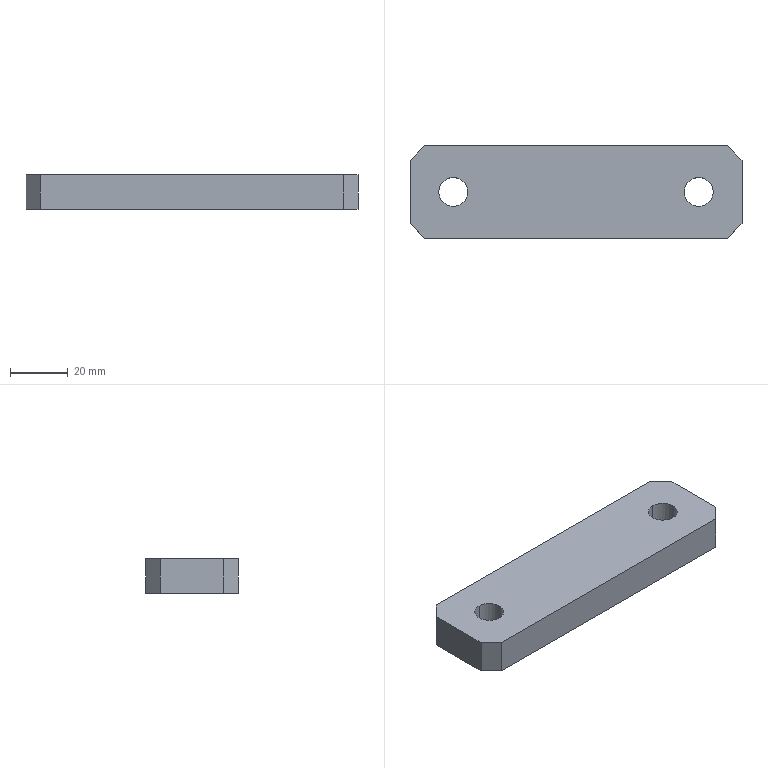Part | STEP file | [23] | 1 solid | 14 faces | box 115 x 32 x 12 mm | volume 41675 mm3 | plane 10 | cylinder 4 | commonest cylinder face diameters 10 x4
STEP:
#1=CARTESIAN_POINT('',(61.,21.,12.));
#2=VERTEX_POINT('',#1);
#3=CARTESIAN_POINT('',(61.,11.,12.));
#4=VERTEX_POINT('',#3);
#5=CARTESIAN_POINT('',(61.,16.,12.));
#6=DIRECTION('',(0.,0.,-1.));
#7=DIRECTION('',(0.,-1.,0.));
#8=AXIS2_PLACEMENT_3D('',#5,#6,#7);
#9=CIRCLE('',#8,5.);
#10=EDGE_CURVE('',#2,#4,#9,.T.);
#11=ORIENTED_EDGE('',*,*,#10,.F.);
#12=CARTESIAN_POINT('',(61.,21.,0.));
#13=VERTEX_POINT('',#12);
#14=CARTESIAN_POINT('',(61.,21.,12.));
#15=DIRECTION('',(0.,0.,-1.));
#16=VECTOR('',#15,1000.);
#17=LINE('',#14,#16);
#18=EDGE_CURVE('',#2,#13,#17,.T.);
#19=ORIENTED_EDGE('',*,*,#18,.T.);
#20=CARTESIAN_POINT('',(61.,11.,0.));
#21=VERTEX_POINT('',#20);
#22=CARTESIAN_POINT('',(61.,16.,0.));
#23=DIRECTION('',(0.,0.,1.));
#24=DIRECTION('',(0.,1.,0.));
#25=AXIS2_PLACEMENT_3D('',#22,#23,#24);
#26=CIRCLE('',#25,5.);
#27=EDGE_CURVE('',#21,#13,#26,.T.);
#28=ORIENTED_EDGE('',*,*,#27,.F.);
#29=CARTESIAN_POINT('',(61.,11.,12.));
#30=DIRECTION('',(0.,0.,-1.));
#31=VECTOR('',#30,1000.);
#32=LINE('',#29,#31);
#33=EDGE_CURVE('',#4,#21,#32,.T.);
#34=ORIENTED_EDGE('',*,*,#33,.F.);
#35=EDGE_LOOP('',(#11,#19,#28,#34));
#36=FACE_OUTER_BOUND('',#35,.T.);
#37=CARTESIAN_POINT('',(61.,16.,12.));
#38=DIRECTION('',(0.,0.,-1.));
#39=DIRECTION('',(0.,-1.,0.));
#40=AXIS2_PLACEMENT_3D('',#37,#38,#39);
#41=CYLINDRICAL_SURFACE('',#40,5.);
#42=ADVANCED_FACE('',(#36),#41,.F.);
#43=CARTESIAN_POINT('',(-24.,21.,12.));
#44=VERTEX_POINT('',#43);
#45=CARTESIAN_POINT('',(-24.,11.,12.));
#46=VERTEX_POINT('',#45);
#47=CARTESIAN_POINT('',(-24.,16.,12.));
#48=DIRECTION('',(0.,0.,-1.));
#49=DIRECTION('',(0.,-1.,0.));
#50=AXIS2_PLACEMENT_3D('',#47,#48,#49);
#51=CIRCLE('',#50,5.);
#52=EDGE_CURVE('',#44,#46,#51,.T.);
#53=ORIENTED_EDGE('',*,*,#52,.F.);
#54=CARTESIAN_POINT('',(-24.,21.,0.));
#55=VERTEX_POINT('',#54);
#56=CARTESIAN_POINT('',(-24.,21.,12.));
#57=DIRECTION('',(0.,0.,-1.));
#58=VECTOR('',#57,1000.);
#59=LINE('',#56,#58);
#60=EDGE_CURVE('',#44,#55,#59,.T.);
#61=ORIENTED_EDGE('',*,*,#60,.T.);
#62=CARTESIAN_POINT('',(-24.,11.,0.));
#63=VERTEX_POINT('',#62);
#64=CARTESIAN_POINT('',(-24.,16.,0.));
#65=DIRECTION('',(0.,0.,1.));
#66=DIRECTION('',(0.,1.,0.));
#67=AXIS2_PLACEMENT_3D('',#64,#65,#66);
#68=CIRCLE('',#67,5.);
#69=EDGE_CURVE('',#63,#55,#68,.T.);
#70=ORIENTED_EDGE('',*,*,#69,.F.);
#71=CARTESIAN_POINT('',(-24.,11.,12.));
#72=DIRECTION('',(0.,0.,-1.));
#73=VECTOR('',#72,1000.);
#74=LINE('',#71,#73);
#75=EDGE_CURVE('',#46,#63,#74,.T.);
#76=ORIENTED_EDGE('',*,*,#75,.F.);
#77=EDGE_LOOP('',(#53,#61,#70,#76));
#78=FACE_OUTER_BOUND('',#77,.T.);
#79=CARTESIAN_POINT('',(-24.,16.,12.));
#80=DIRECTION('',(0.,0.,-1.));
#81=DIRECTION('',(0.,-1.,0.));
#82=AXIS2_PLACEMENT_3D('',#79,#80,#81);
#83=CYLINDRICAL_SURFACE('',#82,5.);
#84=ADVANCED_FACE('',(#78),#83,.F.);
#85=CARTESIAN_POINT('',(61.,16.,12.));
#86=DIRECTION('',(0.,0.,-1.));
#87=DIRECTION('',(0.,-1.,0.));
#88=AXIS2_PLACEMENT_3D('',#85,#86,#87);
#89=CIRCLE('',#88,5.);
#90=EDGE_CURVE('',#4,#2,#89,.T.);
#91=ORIENTED_EDGE('',*,*,#90,.T.);
#92=ORIENTED_EDGE('',*,*,#10,.T.);
#93=EDGE_LOOP('',(#91,#92));
#94=FACE_BOUND('',#93,.T.);
#95=CARTESIAN_POINT('',(-24.,16.,12.));
#96=DIRECTION('',(0.,0.,-1.));
#97=DIRECTION('',(0.,-1.,0.));
#98=AXIS2_PLACEMENT_3D('',#95,#96,#97);
#99=CIRCLE('',#98,5.);
#100=EDGE_CURVE('',#46,#44,#99,.T.);
#101=ORIENTED_EDGE('',*,*,#100,.T.);
#102=ORIENTED_EDGE('',*,*,#52,.T.);
#103=EDGE_LOOP('',(#101,#102));
#104=FACE_BOUND('',#103,.T.);
#105=CARTESIAN_POINT('',(71.,0.,12.));
#106=VERTEX_POINT('',#105);
#107=CARTESIAN_POINT('',(-34.,0.,12.));
#108=VERTEX_POINT('',#107);
#109=CARTESIAN_POINT('',(18.5,0.,12.));
#110=DIRECTION('',(-1.,0.,0.));
#111=VECTOR('',#110,1000.);
#112=LINE('',#109,#111);
#113=EDGE_CURVE('',#106,#108,#112,.T.);
#114=ORIENTED_EDGE('',*,*,#113,.F.);
#115=CARTESIAN_POINT('',(76.,5.,12.));
#116=VERTEX_POINT('',#115);
#117=CARTESIAN_POINT('',(52.75,-18.25,12.));
#118=DIRECTION('',(0.7071,0.7071,0.));
#119=VECTOR('',#118,1000.);
#120=LINE('',#117,#119);
#121=EDGE_CURVE('',#106,#116,#120,.T.);
#122=ORIENTED_EDGE('',*,*,#121,.T.);
#123=CARTESIAN_POINT('',(76.,27.,12.));
#124=VERTEX_POINT('',#123);
#125=CARTESIAN_POINT('',(76.,16.,12.));
#126=DIRECTION('',(0.,-1.,0.));
#127=VECTOR('',#126,1000.);
#128=LINE('',#125,#127);
#129=EDGE_CURVE('',#124,#116,#128,.T.);
#130=ORIENTED_EDGE('',*,*,#129,.F.);
#131=CARTESIAN_POINT('',(71.,32.,12.));
#132=VERTEX_POINT('',#131);
#133=CARTESIAN_POINT('',(52.75,50.25,12.));
#134=DIRECTION('',(-0.7071,0.7071,0.));
#135=VECTOR('',#134,1000.);
#136=LINE('',#133,#135);
#137=EDGE_CURVE('',#124,#132,#136,.T.);
#138=ORIENTED_EDGE('',*,*,#137,.T.);
#139=CARTESIAN_POINT('',(-34.,32.,12.));
#140=VERTEX_POINT('',#139);
#141=CARTESIAN_POINT('',(18.5,32.,12.));
#142=DIRECTION('',(1.,0.,0.));
#143=VECTOR('',#142,1000.);
#144=LINE('',#141,#143);
#145=EDGE_CURVE('',#140,#132,#144,.T.);
#146=ORIENTED_EDGE('',*,*,#145,.F.);
#147=CARTESIAN_POINT('',(-39.,27.,12.));
#148=VERTEX_POINT('',#147);
#149=CARTESIAN_POINT('',(-15.75,50.25,12.));
#150=DIRECTION('',(-0.7071,-0.7071,0.));
#151=VECTOR('',#150,1000.);
#152=LINE('',#149,#151);
#153=EDGE_CURVE('',#140,#148,#152,.T.);
#154=ORIENTED_EDGE('',*,*,#153,.T.);
#155=CARTESIAN_POINT('',(-39.,5.,12.));
#156=VERTEX_POINT('',#155);
#157=CARTESIAN_POINT('',(-39.,16.,12.));
#158=DIRECTION('',(0.,1.,0.));
#159=VECTOR('',#158,1000.);
#160=LINE('',#157,#159);
#161=EDGE_CURVE('',#156,#148,#160,.T.);
#162=ORIENTED_EDGE('',*,*,#161,.F.);
#163=CARTESIAN_POINT('',(-15.75,-18.25,12.));
#164=DIRECTION('',(0.7071,-0.7071,0.));
#165=VECTOR('',#164,1000.);
#166=LINE('',#163,#165);
#167=EDGE_CURVE('',#156,#108,#166,.T.);
#168=ORIENTED_EDGE('',*,*,#167,.T.);
#169=EDGE_LOOP('',(#114,#122,#130,#138,#146,#154,#162,#168));
#170=FACE_OUTER_BOUND('',#169,.T.);
#171=CARTESIAN_POINT('',(18.5,16.,12.));
#172=DIRECTION('',(0.,0.,1.));
#173=DIRECTION('',(0.,1.,0.));
#174=AXIS2_PLACEMENT_3D('',#171,#172,#173);
#175=PLANE('',#174);
#176=ADVANCED_FACE('',(#94,#104,#170),#175,.T.);
#177=ORIENTED_EDGE('',*,*,#129,.T.);
#178=CARTESIAN_POINT('',(76.,5.,0.));
#179=VERTEX_POINT('',#178);
#180=CARTESIAN_POINT('',(76.,5.,0.));
#181=DIRECTION('',(0.,0.,-1.));
#182=VECTOR('',#181,1000.);
#183=LINE('',#180,#182);
#184=EDGE_CURVE('',#116,#179,#183,.T.);
#185=ORIENTED_EDGE('',*,*,#184,.T.);
#186=CARTESIAN_POINT('',(76.,27.,0.));
#187=VERTEX_POINT('',#186);
#188=CARTESIAN_POINT('',(76.,16.,0.));
#189=DIRECTION('',(0.,1.,0.));
#190=VECTOR('',#189,1000.);
#191=LINE('',#188,#190);
#192=EDGE_CURVE('',#179,#187,#191,.T.);
#193=ORIENTED_EDGE('',*,*,#192,.T.);
#194=CARTESIAN_POINT('',(76.,27.,0.));
#195=DIRECTION('',(0.,0.,1.));
#196=VECTOR('',#195,1000.);
#197=LINE('',#194,#196);
#198=EDGE_CURVE('',#187,#124,#197,.T.);
#199=ORIENTED_EDGE('',*,*,#198,.T.);
#200=EDGE_LOOP('',(#177,#185,#193,#199));
#201=FACE_OUTER_BOUND('',#200,.T.);
#202=CARTESIAN_POINT('',(76.,16.,0.));
#203=DIRECTION('',(1.,0.,0.));
#204=DIRECTION('',(0.,0.,-1.));
#205=AXIS2_PLACEMENT_3D('',#202,#203,#204);
#206=PLANE('',#205);
#207=ADVANCED_FACE('',(#201),#206,.T.);
#208=CARTESIAN_POINT('',(-34.,0.,0.));
#209=VERTEX_POINT('',#208);
#210=CARTESIAN_POINT('',(71.,0.,0.));
#211=VERTEX_POINT('',#210);
#212=CARTESIAN_POINT('',(18.5,0.,0.));
#213=DIRECTION('',(1.,0.,0.));
#214=VECTOR('',#213,1000.);
#215=LINE('',#212,#214);
#216=EDGE_CURVE('',#209,#211,#215,.T.);
#217=ORIENTED_EDGE('',*,*,#216,.T.);
#218=CARTESIAN_POINT('',(71.,0.,0.));
#219=DIRECTION('',(0.,0.,1.));
#220=VECTOR('',#219,1000.);
#221=LINE('',#218,#220);
#222=EDGE_CURVE('',#211,#106,#221,.T.);
#223=ORIENTED_EDGE('',*,*,#222,.T.);
#224=ORIENTED_EDGE('',*,*,#113,.T.);
#225=CARTESIAN_POINT('',(-34.,0.,0.));
#226=DIRECTION('',(0.,0.,-1.));
#227=VECTOR('',#226,1000.);
#228=LINE('',#225,#227);
#229=EDGE_CURVE('',#108,#209,#228,.T.);
#230=ORIENTED_EDGE('',*,*,#229,.T.);
#231=EDGE_LOOP('',(#217,#223,#224,#230));
#232=FACE_OUTER_BOUND('',#231,.T.);
#233=CARTESIAN_POINT('',(18.5,0.,0.));
#234=DIRECTION('',(0.,-1.,0.));
#235=DIRECTION('',(0.,0.,1.));
#236=AXIS2_PLACEMENT_3D('',#233,#234,#235);
#237=PLANE('',#236);
#238=ADVANCED_FACE('',(#232),#237,.T.);
#239=ORIENTED_EDGE('',*,*,#161,.T.);
#240=CARTESIAN_POINT('',(-39.,27.,0.));
#241=VERTEX_POINT('',#240);
#242=CARTESIAN_POINT('',(-39.,27.,0.));
#243=DIRECTION('',(0.,0.,-1.));
#244=VECTOR('',#243,1000.);
#245=LINE('',#242,#244);
#246=EDGE_CURVE('',#148,#241,#245,.T.);
#247=ORIENTED_EDGE('',*,*,#246,.T.);
#248=CARTESIAN_POINT('',(-39.,5.,0.));
#249=VERTEX_POINT('',#248);
#250=CARTESIAN_POINT('',(-39.,16.,0.));
#251=DIRECTION('',(0.,-1.,0.));
#252=VECTOR('',#251,1000.);
#253=LINE('',#250,#252);
#254=EDGE_CURVE('',#241,#249,#253,.T.);
#255=ORIENTED_EDGE('',*,*,#254,.T.);
#256=CARTESIAN_POINT('',(-39.,5.,0.));
#257=DIRECTION('',(0.,0.,1.));
#258=VECTOR('',#257,1000.);
#259=LINE('',#256,#258);
#260=EDGE_CURVE('',#249,#156,#259,.T.);
#261=ORIENTED_EDGE('',*,*,#260,.T.);
#262=EDGE_LOOP('',(#239,#247,#255,#261));
#263=FACE_OUTER_BOUND('',#262,.T.);
#264=CARTESIAN_POINT('',(-39.,16.,0.));
#265=DIRECTION('',(-1.,0.,0.));
#266=DIRECTION('',(0.,0.,1.));
#267=AXIS2_PLACEMENT_3D('',#264,#265,#266);
#268=PLANE('',#267);
#269=ADVANCED_FACE('',(#263),#268,.T.);
#270=ORIENTED_EDGE('',*,*,#27,.T.);
#271=CARTESIAN_POINT('',(61.,16.,0.));
#272=DIRECTION('',(0.,0.,1.));
#273=DIRECTION('',(0.,1.,0.));
#274=AXIS2_PLACEMENT_3D('',#271,#272,#273);
#275=CIRCLE('',#274,5.);
#276=EDGE_CURVE('',#13,#21,#275,.T.);
#277=ORIENTED_EDGE('',*,*,#276,.T.);
#278=EDGE_LOOP('',(#270,#277));
#279=FACE_BOUND('',#278,.T.);
#280=ORIENTED_EDGE('',*,*,#69,.T.);
#281=CARTESIAN_POINT('',(-24.,16.,0.));
#282=DIRECTION('',(0.,0.,1.));
#283=DIRECTION('',(0.,1.,0.));
#284=AXIS2_PLACEMENT_3D('',#281,#282,#283);
#285=CIRCLE('',#284,5.);
#286=EDGE_CURVE('',#55,#63,#285,.T.);
#287=ORIENTED_EDGE('',*,*,#286,.T.);
#288=EDGE_LOOP('',(#280,#287));
#289=FACE_BOUND('',#288,.T.);
#290=ORIENTED_EDGE('',*,*,#192,.F.);
#291=CARTESIAN_POINT('',(52.75,-18.25,0.));
#292=DIRECTION('',(-0.7071,-0.7071,0.));
#293=VECTOR('',#292,1000.);
#294=LINE('',#291,#293);
#295=EDGE_CURVE('',#179,#211,#294,.T.);
#296=ORIENTED_EDGE('',*,*,#295,.T.);
#297=ORIENTED_EDGE('',*,*,#216,.F.);
#298=CARTESIAN_POINT('',(-15.75,-18.25,0.));
#299=DIRECTION('',(-0.7071,0.7071,0.));
#300=VECTOR('',#299,1000.);
#301=LINE('',#298,#300);
#302=EDGE_CURVE('',#209,#249,#301,.T.);
#303=ORIENTED_EDGE('',*,*,#302,.T.);
#304=ORIENTED_EDGE('',*,*,#254,.F.);
#305=CARTESIAN_POINT('',(-34.,32.,0.));
#306=VERTEX_POINT('',#305);
#307=CARTESIAN_POINT('',(-15.75,50.25,0.));
#308=DIRECTION('',(0.7071,0.7071,0.));
#309=VECTOR('',#308,1000.);
#310=LINE('',#307,#309);
#311=EDGE_CURVE('',#241,#306,#310,.T.);
#312=ORIENTED_EDGE('',*,*,#311,.T.);
#313=CARTESIAN_POINT('',(71.,32.,0.));
#314=VERTEX_POINT('',#313);
#315=CARTESIAN_POINT('',(18.5,32.,0.));
#316=DIRECTION('',(-1.,0.,0.));
#317=VECTOR('',#316,1000.);
#318=LINE('',#315,#317);
#319=EDGE_CURVE('',#314,#306,#318,.T.);
#320=ORIENTED_EDGE('',*,*,#319,.F.);
#321=CARTESIAN_POINT('',(52.75,50.25,0.));
#322=DIRECTION('',(0.7071,-0.7071,0.));
#323=VECTOR('',#322,1000.);
#324=LINE('',#321,#323);
#325=EDGE_CURVE('',#314,#187,#324,.T.);
#326=ORIENTED_EDGE('',*,*,#325,.T.);
#327=EDGE_LOOP('',(#290,#296,#297,#303,#304,#312,#320,#326));
#328=FACE_OUTER_BOUND('',#327,.T.);
#329=CARTESIAN_POINT('',(18.5,16.,0.));
#330=DIRECTION('',(0.,0.,-1.));
#331=DIRECTION('',(0.,-1.,0.));
#332=AXIS2_PLACEMENT_3D('',#329,#330,#331);
#333=PLANE('',#332);
#334=ADVANCED_FACE('',(#279,#289,#328),#333,.T.);
#335=ORIENTED_EDGE('',*,*,#145,.T.);
#336=CARTESIAN_POINT('',(71.,32.,0.));
#337=DIRECTION('',(0.,0.,-1.));
#338=VECTOR('',#337,1000.);
#339=LINE('',#336,#338);
#340=EDGE_CURVE('',#132,#314,#339,.T.);
#341=ORIENTED_EDGE('',*,*,#340,.T.);
#342=ORIENTED_EDGE('',*,*,#319,.T.);
#343=CARTESIAN_POINT('',(-34.,32.,0.));
#344=DIRECTION('',(0.,0.,1.));
#345=VECTOR('',#344,1000.);
#346=LINE('',#343,#345);
#347=EDGE_CURVE('',#306,#140,#346,.T.);
#348=ORIENTED_EDGE('',*,*,#347,.T.);
#349=EDGE_LOOP('',(#335,#341,#342,#348));
#350=FACE_OUTER_BOUND('',#349,.T.);
#351=CARTESIAN_POINT('',(18.5,32.,0.));
#352=DIRECTION('',(0.,1.,0.));
#353=DIRECTION('',(0.,0.,-1.));
#354=AXIS2_PLACEMENT_3D('',#351,#352,#353);
#355=PLANE('',#354);
#356=ADVANCED_FACE('',(#350),#355,.T.);
#357=ORIENTED_EDGE('',*,*,#302,.F.);
#358=ORIENTED_EDGE('',*,*,#229,.F.);
#359=ORIENTED_EDGE('',*,*,#167,.F.);
#360=ORIENTED_EDGE('',*,*,#260,.F.);
#361=EDGE_LOOP('',(#357,#358,#359,#360));
#362=FACE_OUTER_BOUND('',#361,.T.);
#363=CARTESIAN_POINT('',(-39.,5.,0.));
#364=DIRECTION('',(0.7071,0.7071,0.));
#365=DIRECTION('',(0.,0.,1.));
#366=AXIS2_PLACEMENT_3D('',#363,#364,#365);
#367=PLANE('',#366);
#368=ADVANCED_FACE('',(#362),#367,.F.);
#369=ORIENTED_EDGE('',*,*,#311,.F.);
#370=ORIENTED_EDGE('',*,*,#246,.F.);
#371=ORIENTED_EDGE('',*,*,#153,.F.);
#372=ORIENTED_EDGE('',*,*,#347,.F.);
#373=EDGE_LOOP('',(#369,#370,#371,#372));
#374=FACE_OUTER_BOUND('',#373,.T.);
#375=CARTESIAN_POINT('',(-34.,32.,0.));
#376=DIRECTION('',(0.7071,-0.7071,0.));
#377=DIRECTION('',(0.,0.,1.));
#378=AXIS2_PLACEMENT_3D('',#375,#376,#377);
#379=PLANE('',#378);
#380=ADVANCED_FACE('',(#374),#379,.F.);
#381=ORIENTED_EDGE('',*,*,#325,.F.);
#382=ORIENTED_EDGE('',*,*,#340,.F.);
#383=ORIENTED_EDGE('',*,*,#137,.F.);
#384=ORIENTED_EDGE('',*,*,#198,.F.);
#385=EDGE_LOOP('',(#381,#382,#383,#384));
#386=FACE_OUTER_BOUND('',#385,.T.);
#387=CARTESIAN_POINT('',(76.,27.,0.));
#388=DIRECTION('',(-0.7071,-0.7071,0.));
#389=DIRECTION('',(0.,0.,1.));
#390=AXIS2_PLACEMENT_3D('',#387,#388,#389);
#391=PLANE('',#390);
#392=ADVANCED_FACE('',(#386),#391,.F.);
#393=ORIENTED_EDGE('',*,*,#295,.F.);
#394=ORIENTED_EDGE('',*,*,#184,.F.);
#395=ORIENTED_EDGE('',*,*,#121,.F.);
#396=ORIENTED_EDGE('',*,*,#222,.F.);
#397=EDGE_LOOP('',(#393,#394,#395,#396));
#398=FACE_OUTER_BOUND('',#397,.T.);
#399=CARTESIAN_POINT('',(71.,0.,0.));
#400=DIRECTION('',(-0.7071,0.7071,0.));
#401=DIRECTION('',(0.,0.,1.));
#402=AXIS2_PLACEMENT_3D('',#399,#400,#401);
#403=PLANE('',#402);
#404=ADVANCED_FACE('',(#398),#403,.F.);
#405=ORIENTED_EDGE('',*,*,#60,.F.);
#406=ORIENTED_EDGE('',*,*,#100,.F.);
#407=ORIENTED_EDGE('',*,*,#75,.T.);
#408=ORIENTED_EDGE('',*,*,#286,.F.);
#409=EDGE_LOOP('',(#405,#406,#407,#408));
#410=FACE_OUTER_BOUND('',#409,.T.);
#411=CARTESIAN_POINT('',(-24.,16.,12.));
#412=DIRECTION('',(0.,0.,-1.));
#413=DIRECTION('',(0.,-1.,0.));
#414=AXIS2_PLACEMENT_3D('',#411,#412,#413);
#415=CYLINDRICAL_SURFACE('',#414,5.);
#416=ADVANCED_FACE('',(#410),#415,.F.);
#417=ORIENTED_EDGE('',*,*,#18,.F.);
#418=ORIENTED_EDGE('',*,*,#90,.F.);
#419=ORIENTED_EDGE('',*,*,#33,.T.);
#420=ORIENTED_EDGE('',*,*,#276,.F.);
#421=EDGE_LOOP('',(#417,#418,#419,#420));
#422=FACE_OUTER_BOUND('',#421,.T.);
#423=CARTESIAN_POINT('',(61.,16.,12.));
#424=DIRECTION('',(0.,0.,-1.));
#425=DIRECTION('',(0.,-1.,0.));
#426=AXIS2_PLACEMENT_3D('',#423,#424,#425);
#427=CYLINDRICAL_SURFACE('',#426,5.);
#428=ADVANCED_FACE('',(#422),#427,.F.);
#429=CLOSED_SHELL('',(#42,#84,#176,#207,#238,#269,#334,#356,#368,#380,#392,#404,#416,#428));
#430=MANIFOLD_SOLID_BREP('',#429);
#431=CARTESIAN_POINT('',(0.,0.,0.));
#432=DIRECTION('',(0.,0.,1.));
#433=DIRECTION('',(1.,0.,0.));
#434=AXIS2_PLACEMENT_3D('',#431,#432,#433);
#435=(LENGTH_UNIT()NAMED_UNIT(*)SI_UNIT(.MILLI.,.METRE.));
#436=UNCERTAINTY_MEASURE_WITH_UNIT(LENGTH_MEASURE(0.00001),#435,'','');
#437=(NAMED_UNIT(*)PLANE_ANGLE_UNIT()SI_UNIT($,.RADIAN.));
#438=(NAMED_UNIT(*)SI_UNIT($,.STERADIAN.)SOLID_ANGLE_UNIT());
#439=(GEOMETRIC_REPRESENTATION_CONTEXT(3)GLOBAL_UNCERTAINTY_ASSIGNED_CONTEXT((#436))GLOBAL_UNIT_ASSIGNED_CONTEXT((#435,#437,#438))REPRESENTATION_CONTEXT('',''));
#440=ADVANCED_BREP_SHAPE_REPRESENTATION('',(#430,#434),#439);